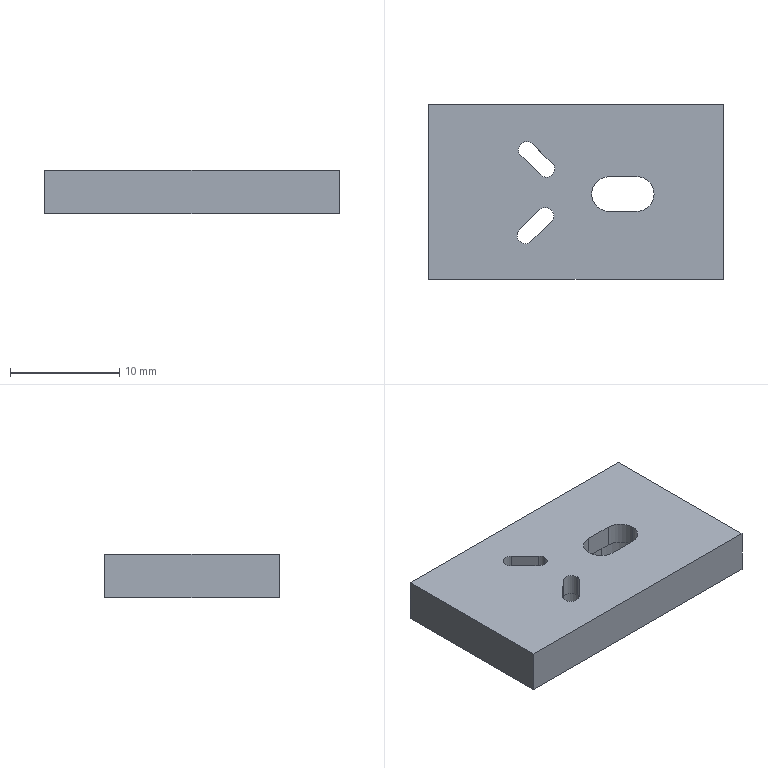Part | SolidWorks | features Cut 2, Extrusion 1, ICE 1 | 1 solid | 39 faces | box 27 x 16 x 4 mm | volume 1564 mm3 | plane 21 | cylinder 18 | commonest cylinder face diameters 1.5 x6 2.5 x6 3.18 x3 5 x3
STEP:
#1=CARTESIAN_POINT('',(4.433,-4.071,2.));
#2=VERTEX_POINT('',#1);
#3=CARTESIAN_POINT('',(6.931,-1.571,2.));
#4=VERTEX_POINT('',#3);
#5=CARTESIAN_POINT('',(6.933,-4.071,2.));
#6=DIRECTION('',(0.,0.,-1.));
#7=DIRECTION('',(-1.,0.,0.));
#8=AXIS2_PLACEMENT_3D('',#5,#6,#7);
#9=CIRCLE('',#8,2.5);
#10=EDGE_CURVE('',#2,#4,#9,.T.);
#11=ORIENTED_EDGE('',*,*,#10,.F.);
#12=CARTESIAN_POINT('',(4.433,-4.071,0.));
#13=VERTEX_POINT('',#12);
#14=CARTESIAN_POINT('',(4.433,-4.071,2.));
#15=DIRECTION('',(0.,0.,-1.));
#16=VECTOR('',#15,1000.);
#17=LINE('',#14,#16);
#18=EDGE_CURVE('',#2,#13,#17,.T.);
#19=ORIENTED_EDGE('',*,*,#18,.T.);
#20=CARTESIAN_POINT('',(6.931,-1.571,0.));
#21=VERTEX_POINT('',#20);
#22=CARTESIAN_POINT('',(6.933,-4.071,0.));
#23=DIRECTION('',(0.,0.,-1.));
#24=DIRECTION('',(-1.,0.,0.));
#25=AXIS2_PLACEMENT_3D('',#22,#23,#24);
#26=CIRCLE('',#25,2.5);
#27=EDGE_CURVE('',#13,#21,#26,.T.);
#28=ORIENTED_EDGE('',*,*,#27,.T.);
#29=CARTESIAN_POINT('',(6.931,-1.571,2.));
#30=DIRECTION('',(0.,0.,-1.));
#31=VECTOR('',#30,1000.);
#32=LINE('',#29,#31);
#33=EDGE_CURVE('',#4,#21,#32,.T.);
#34=ORIENTED_EDGE('',*,*,#33,.F.);
#35=EDGE_LOOP('',(#11,#19,#28,#34));
#36=FACE_OUTER_BOUND('',#35,.T.);
#37=CARTESIAN_POINT('',(6.933,-4.071,2.));
#38=DIRECTION('',(0.,0.,-1.));
#39=DIRECTION('',(-1.,0.,0.));
#40=AXIS2_PLACEMENT_3D('',#37,#38,#39);
#41=CYLINDRICAL_SURFACE('',#40,2.5);
#42=ADVANCED_FACE('',(#36),#41,.F.);
#43=CARTESIAN_POINT('',(-2.005,-7.872,2.));
#44=VERTEX_POINT('',#43);
#45=CARTESIAN_POINT('',(-1.624,-6.973,2.));
#46=VERTEX_POINT('',#45);
#47=CARTESIAN_POINT('',(-0.7552,-7.872,2.));
#48=DIRECTION('',(0.,0.,-1.));
#49=DIRECTION('',(-1.,0.,0.));
#50=AXIS2_PLACEMENT_3D('',#47,#48,#49);
#51=CIRCLE('',#50,1.25);
#52=EDGE_CURVE('',#44,#46,#51,.T.);
#53=ORIENTED_EDGE('',*,*,#52,.F.);
#54=CARTESIAN_POINT('',(-2.005,-7.872,0.));
#55=VERTEX_POINT('',#54);
#56=CARTESIAN_POINT('',(-2.005,-7.872,2.));
#57=DIRECTION('',(0.,0.,-1.));
#58=VECTOR('',#57,1000.);
#59=LINE('',#56,#58);
#60=EDGE_CURVE('',#44,#55,#59,.T.);
#61=ORIENTED_EDGE('',*,*,#60,.T.);
#62=CARTESIAN_POINT('',(-1.624,-6.973,0.));
#63=VERTEX_POINT('',#62);
#64=CARTESIAN_POINT('',(-0.7552,-7.872,0.));
#65=DIRECTION('',(0.,0.,-1.));
#66=DIRECTION('',(-1.,0.,0.));
#67=AXIS2_PLACEMENT_3D('',#64,#65,#66);
#68=CIRCLE('',#67,1.25);
#69=EDGE_CURVE('',#55,#63,#68,.T.);
#70=ORIENTED_EDGE('',*,*,#69,.T.);
#71=CARTESIAN_POINT('',(-1.624,-6.973,2.));
#72=DIRECTION('',(0.,0.,-1.));
#73=VECTOR('',#72,1000.);
#74=LINE('',#71,#73);
#75=EDGE_CURVE('',#46,#63,#74,.T.);
#76=ORIENTED_EDGE('',*,*,#75,.F.);
#77=EDGE_LOOP('',(#53,#61,#70,#76));
#78=FACE_OUTER_BOUND('',#77,.T.);
#79=CARTESIAN_POINT('',(-0.7552,-7.872,2.));
#80=DIRECTION('',(0.,0.,-1.));
#81=DIRECTION('',(-1.,0.,0.));
#82=AXIS2_PLACEMENT_3D('',#79,#80,#81);
#83=CYLINDRICAL_SURFACE('',#82,1.25);
#84=ADVANCED_FACE('',(#78),#83,.F.);
#85=CARTESIAN_POINT('',(-1.875,-0.01768,2.));
#86=VERTEX_POINT('',#85);
#87=CARTESIAN_POINT('',(0.2441,0.881,2.));
#88=VERTEX_POINT('',#87);
#89=CARTESIAN_POINT('',(-0.6247,-0.01768,2.));
#90=DIRECTION('',(0.,0.,-1.));
#91=DIRECTION('',(-1.,0.,0.));
#92=AXIS2_PLACEMENT_3D('',#89,#90,#91);
#93=CIRCLE('',#92,1.25);
#94=EDGE_CURVE('',#86,#88,#93,.T.);
#95=ORIENTED_EDGE('',*,*,#94,.F.);
#96=CARTESIAN_POINT('',(-1.875,-0.01768,0.));
#97=VERTEX_POINT('',#96);
#98=CARTESIAN_POINT('',(-1.875,-0.01768,2.));
#99=DIRECTION('',(0.,0.,-1.));
#100=VECTOR('',#99,1000.);
#101=LINE('',#98,#100);
#102=EDGE_CURVE('',#86,#97,#101,.T.);
#103=ORIENTED_EDGE('',*,*,#102,.T.);
#104=CARTESIAN_POINT('',(0.2441,0.881,0.));
#105=VERTEX_POINT('',#104);
#106=CARTESIAN_POINT('',(-0.6247,-0.01768,0.));
#107=DIRECTION('',(0.,0.,-1.));
#108=DIRECTION('',(-1.,0.,0.));
#109=AXIS2_PLACEMENT_3D('',#106,#107,#108);
#110=CIRCLE('',#109,1.25);
#111=EDGE_CURVE('',#97,#105,#110,.T.);
#112=ORIENTED_EDGE('',*,*,#111,.T.);
#113=CARTESIAN_POINT('',(0.2441,0.881,2.));
#114=DIRECTION('',(0.,0.,-1.));
#115=VECTOR('',#114,1000.);
#116=LINE('',#113,#115);
#117=EDGE_CURVE('',#88,#105,#116,.T.);
#118=ORIENTED_EDGE('',*,*,#117,.F.);
#119=EDGE_LOOP('',(#95,#103,#112,#118));
#120=FACE_OUTER_BOUND('',#119,.T.);
#121=CARTESIAN_POINT('',(-0.6247,-0.01768,2.));
#122=DIRECTION('',(0.,0.,-1.));
#123=DIRECTION('',(-1.,0.,0.));
#124=AXIS2_PLACEMENT_3D('',#121,#122,#123);
#125=CYLINDRICAL_SURFACE('',#124,1.25);
#126=ADVANCED_FACE('',(#120),#125,.F.);
#127=CARTESIAN_POINT('',(11.055,-4.07,2.));
#128=VERTEX_POINT('',#127);
#129=CARTESIAN_POINT('',(9.464,-2.48,2.));
#130=VERTEX_POINT('',#129);
#131=CARTESIAN_POINT('',(9.465,-4.07,2.));
#132=DIRECTION('',(0.,0.,1.));
#133=DIRECTION('',(-1.,0.,0.));
#134=AXIS2_PLACEMENT_3D('',#131,#132,#133);
#135=CIRCLE('',#134,1.59);
#136=EDGE_CURVE('',#128,#130,#135,.T.);
#137=ORIENTED_EDGE('',*,*,#136,.F.);
#138=CARTESIAN_POINT('',(11.055,-4.07,4.));
#139=VERTEX_POINT('',#138);
#140=CARTESIAN_POINT('',(11.055,-4.07,-4.497));
#141=DIRECTION('',(0.,0.,1.));
#142=VECTOR('',#141,1000.);
#143=LINE('',#140,#142);
#144=EDGE_CURVE('',#128,#139,#143,.T.);
#145=ORIENTED_EDGE('',*,*,#144,.T.);
#146=CARTESIAN_POINT('',(9.464,-2.48,4.));
#147=VERTEX_POINT('',#146);
#148=CARTESIAN_POINT('',(9.465,-4.07,4.));
#149=DIRECTION('',(0.,0.,1.));
#150=DIRECTION('',(1.,0.,0.));
#151=AXIS2_PLACEMENT_3D('',#148,#149,#150);
#152=CIRCLE('',#151,1.59);
#153=EDGE_CURVE('',#139,#147,#152,.T.);
#154=ORIENTED_EDGE('',*,*,#153,.T.);
#155=CARTESIAN_POINT('',(9.464,-2.48,-5.208));
#156=DIRECTION('',(0.,0.,1.));
#157=VECTOR('',#156,1000.);
#158=LINE('',#155,#157);
#159=EDGE_CURVE('',#130,#147,#158,.T.);
#160=ORIENTED_EDGE('',*,*,#159,.F.);
#161=EDGE_LOOP('',(#137,#145,#154,#160));
#162=FACE_OUTER_BOUND('',#161,.T.);
#163=CARTESIAN_POINT('',(9.465,-4.07,-4.497));
#164=DIRECTION('',(0.,0.,1.));
#165=DIRECTION('',(1.,0.,0.));
#166=AXIS2_PLACEMENT_3D('',#163,#164,#165);
#167=CYLINDRICAL_SURFACE('',#166,1.59);
#168=ADVANCED_FACE('',(#162),#167,.F.);
#169=CARTESIAN_POINT('',(1.95,-1.782,2.));
#170=VERTEX_POINT('',#169);
#171=CARTESIAN_POINT('',(1.721,-1.242,2.));
#172=VERTEX_POINT('',#171);
#173=CARTESIAN_POINT('',(1.2,-1.782,2.));
#174=DIRECTION('',(0.,0.,1.));
#175=DIRECTION('',(-1.,0.,0.));
#176=AXIS2_PLACEMENT_3D('',#173,#174,#175);
#177=CIRCLE('',#176,0.75);
#178=EDGE_CURVE('',#170,#172,#177,.T.);
#179=ORIENTED_EDGE('',*,*,#178,.F.);
#180=CARTESIAN_POINT('',(1.95,-1.782,4.));
#181=VERTEX_POINT('',#180);
#182=CARTESIAN_POINT('',(1.95,-1.782,-4.497));
#183=DIRECTION('',(0.,0.,1.));
#184=VECTOR('',#183,1000.);
#185=LINE('',#182,#184);
#186=EDGE_CURVE('',#170,#181,#185,.T.);
#187=ORIENTED_EDGE('',*,*,#186,.T.);
#188=CARTESIAN_POINT('',(1.721,-1.242,4.));
#189=VERTEX_POINT('',#188);
#190=CARTESIAN_POINT('',(1.2,-1.782,4.));
#191=DIRECTION('',(0.,0.,1.));
#192=DIRECTION('',(1.,0.,0.));
#193=AXIS2_PLACEMENT_3D('',#190,#191,#192);
#194=CIRCLE('',#193,0.75);
#195=EDGE_CURVE('',#181,#189,#194,.T.);
#196=ORIENTED_EDGE('',*,*,#195,.T.);
#197=CARTESIAN_POINT('',(1.721,-1.242,-5.208));
#198=DIRECTION('',(0.,0.,1.));
#199=VECTOR('',#198,1000.);
#200=LINE('',#197,#199);
#201=EDGE_CURVE('',#172,#189,#200,.T.);
#202=ORIENTED_EDGE('',*,*,#201,.F.);
#203=EDGE_LOOP('',(#179,#187,#196,#202));
#204=FACE_OUTER_BOUND('',#203,.T.);
#205=CARTESIAN_POINT('',(1.2,-1.782,-4.497));
#206=DIRECTION('',(0.,0.,1.));
#207=DIRECTION('',(1.,0.,0.));
#208=AXIS2_PLACEMENT_3D('',#205,#206,#207);
#209=CYLINDRICAL_SURFACE('',#208,0.75);
#210=ADVANCED_FACE('',(#204),#209,.F.);
#211=CARTESIAN_POINT('',(1.873,-6.057,2.));
#212=VERTEX_POINT('',#211);
#213=CARTESIAN_POINT('',(0.6012,-5.518,2.));
#214=VERTEX_POINT('',#213);
#215=CARTESIAN_POINT('',(1.123,-6.057,2.));
#216=DIRECTION('',(0.,0.,1.));
#217=DIRECTION('',(-1.,0.,0.));
#218=AXIS2_PLACEMENT_3D('',#215,#216,#217);
#219=CIRCLE('',#218,0.75);
#220=EDGE_CURVE('',#212,#214,#219,.T.);
#221=ORIENTED_EDGE('',*,*,#220,.F.);
#222=CARTESIAN_POINT('',(1.873,-6.057,4.));
#223=VERTEX_POINT('',#222);
#224=CARTESIAN_POINT('',(1.873,-6.057,-4.497));
#225=DIRECTION('',(0.,0.,1.));
#226=VECTOR('',#225,1000.);
#227=LINE('',#224,#226);
#228=EDGE_CURVE('',#212,#223,#227,.T.);
#229=ORIENTED_EDGE('',*,*,#228,.T.);
#230=CARTESIAN_POINT('',(0.6012,-5.518,4.));
#231=VERTEX_POINT('',#230);
#232=CARTESIAN_POINT('',(1.123,-6.057,4.));
#233=DIRECTION('',(0.,0.,1.));
#234=DIRECTION('',(1.,0.,0.));
#235=AXIS2_PLACEMENT_3D('',#232,#233,#234);
#236=CIRCLE('',#235,0.75);
#237=EDGE_CURVE('',#223,#231,#236,.T.);
#238=ORIENTED_EDGE('',*,*,#237,.T.);
#239=CARTESIAN_POINT('',(0.6012,-5.518,-5.208));
#240=DIRECTION('',(0.,0.,1.));
#241=VECTOR('',#240,1000.);
#242=LINE('',#239,#241);
#243=EDGE_CURVE('',#214,#231,#242,.T.);
#244=ORIENTED_EDGE('',*,*,#243,.F.);
#245=EDGE_LOOP('',(#221,#229,#238,#244));
#246=FACE_OUTER_BOUND('',#245,.T.);
#247=CARTESIAN_POINT('',(1.123,-6.057,-4.497));
#248=DIRECTION('',(0.,0.,1.));
#249=DIRECTION('',(1.,0.,0.));
#250=AXIS2_PLACEMENT_3D('',#247,#248,#249);
#251=CYLINDRICAL_SURFACE('',#250,0.75);
#252=ADVANCED_FACE('',(#246),#251,.F.);
#253=ORIENTED_EDGE('',*,*,#228,.F.);
#254=CARTESIAN_POINT('',(1.644,-6.596,2.));
#255=VERTEX_POINT('',#254);
#256=CARTESIAN_POINT('',(1.123,-6.057,2.));
#257=DIRECTION('',(0.,0.,1.));
#258=DIRECTION('',(-1.,0.,0.));
#259=AXIS2_PLACEMENT_3D('',#256,#257,#258);
#260=CIRCLE('',#259,0.75);
#261=EDGE_CURVE('',#255,#212,#260,.T.);
#262=ORIENTED_EDGE('',*,*,#261,.F.);
#263=CARTESIAN_POINT('',(1.644,-6.596,4.));
#264=VERTEX_POINT('',#263);
#265=CARTESIAN_POINT('',(1.644,-6.596,-5.208));
#266=DIRECTION('',(0.,0.,1.));
#267=VECTOR('',#266,1000.);
#268=LINE('',#265,#267);
#269=EDGE_CURVE('',#255,#264,#268,.T.);
#270=ORIENTED_EDGE('',*,*,#269,.T.);
#271=CARTESIAN_POINT('',(1.123,-6.057,4.));
#272=DIRECTION('',(0.,0.,1.));
#273=DIRECTION('',(1.,0.,0.));
#274=AXIS2_PLACEMENT_3D('',#271,#272,#273);
#275=CIRCLE('',#274,0.75);
#276=EDGE_CURVE('',#264,#223,#275,.T.);
#277=ORIENTED_EDGE('',*,*,#276,.T.);
#278=EDGE_LOOP('',(#253,#262,#270,#277));
#279=FACE_OUTER_BOUND('',#278,.T.);
#280=CARTESIAN_POINT('',(1.123,-6.057,-4.497));
#281=DIRECTION('',(0.,0.,1.));
#282=DIRECTION('',(1.,0.,0.));
#283=AXIS2_PLACEMENT_3D('',#280,#281,#282);
#284=CYLINDRICAL_SURFACE('',#283,0.75);
#285=ADVANCED_FACE('',(#279),#284,.F.);
#286=ORIENTED_EDGE('',*,*,#186,.F.);
#287=CARTESIAN_POINT('',(0.6786,-2.321,2.));
#288=VERTEX_POINT('',#287);
#289=CARTESIAN_POINT('',(1.2,-1.782,2.));
#290=DIRECTION('',(0.,0.,1.));
#291=DIRECTION('',(-1.,0.,0.));
#292=AXIS2_PLACEMENT_3D('',#289,#290,#291);
#293=CIRCLE('',#292,0.75);
#294=EDGE_CURVE('',#288,#170,#293,.T.);
#295=ORIENTED_EDGE('',*,*,#294,.F.);
#296=CARTESIAN_POINT('',(0.6786,-2.321,4.));
#297=VERTEX_POINT('',#296);
#298=CARTESIAN_POINT('',(0.6786,-2.321,-5.208));
#299=DIRECTION('',(0.,0.,1.));
#300=VECTOR('',#299,1000.);
#301=LINE('',#298,#300);
#302=EDGE_CURVE('',#288,#297,#301,.T.);
#303=ORIENTED_EDGE('',*,*,#302,.T.);
#304=CARTESIAN_POINT('',(1.2,-1.782,4.));
#305=DIRECTION('',(0.,0.,1.));
#306=DIRECTION('',(1.,0.,0.));
#307=AXIS2_PLACEMENT_3D('',#304,#305,#306);
#308=CIRCLE('',#307,0.75);
#309=EDGE_CURVE('',#297,#181,#308,.T.);
#310=ORIENTED_EDGE('',*,*,#309,.T.);
#311=EDGE_LOOP('',(#286,#295,#303,#310));
#312=FACE_OUTER_BOUND('',#311,.T.);
#313=CARTESIAN_POINT('',(1.2,-1.782,-4.497));
#314=DIRECTION('',(0.,0.,1.));
#315=DIRECTION('',(1.,0.,0.));
#316=AXIS2_PLACEMENT_3D('',#313,#314,#315);
#317=CYLINDRICAL_SURFACE('',#316,0.75);
#318=ADVANCED_FACE('',(#312),#317,.F.);
#319=ORIENTED_EDGE('',*,*,#144,.F.);
#320=CARTESIAN_POINT('',(9.467,-5.66,2.));
#321=VERTEX_POINT('',#320);
#322=CARTESIAN_POINT('',(9.465,-4.07,2.));
#323=DIRECTION('',(0.,0.,1.));
#324=DIRECTION('',(-1.,0.,0.));
#325=AXIS2_PLACEMENT_3D('',#322,#323,#324);
#326=CIRCLE('',#325,1.59);
#327=EDGE_CURVE('',#321,#128,#326,.T.);
#328=ORIENTED_EDGE('',*,*,#327,.F.);
#329=CARTESIAN_POINT('',(9.467,-5.66,4.));
#330=VERTEX_POINT('',#329);
#331=CARTESIAN_POINT('',(9.467,-5.66,-5.208));
#332=DIRECTION('',(0.,0.,1.));
#333=VECTOR('',#332,1000.);
#334=LINE('',#331,#333);
#335=EDGE_CURVE('',#321,#330,#334,.T.);
#336=ORIENTED_EDGE('',*,*,#335,.T.);
#337=CARTESIAN_POINT('',(9.465,-4.07,4.));
#338=DIRECTION('',(0.,0.,1.));
#339=DIRECTION('',(1.,0.,0.));
#340=AXIS2_PLACEMENT_3D('',#337,#338,#339);
#341=CIRCLE('',#340,1.59);
#342=EDGE_CURVE('',#330,#139,#341,.T.);
#343=ORIENTED_EDGE('',*,*,#342,.T.);
#344=EDGE_LOOP('',(#319,#328,#336,#343));
#345=FACE_OUTER_BOUND('',#344,.T.);
#346=CARTESIAN_POINT('',(9.465,-4.07,-4.497));
#347=DIRECTION('',(0.,0.,1.));
#348=DIRECTION('',(1.,0.,0.));
#349=AXIS2_PLACEMENT_3D('',#346,#347,#348);
#350=CYLINDRICAL_SURFACE('',#349,1.59);
#351=ADVANCED_FACE('',(#345),#350,.F.);
#352=CARTESIAN_POINT('',(6.932,-2.481,2.));
#353=VERTEX_POINT('',#352);
#354=CARTESIAN_POINT('',(6.934,-5.661,2.));
#355=VERTEX_POINT('',#354);
#356=CARTESIAN_POINT('',(6.933,-4.071,2.));
#357=DIRECTION('',(0.,0.,1.));
#358=DIRECTION('',(-1.,0.,0.));
#359=AXIS2_PLACEMENT_3D('',#356,#357,#358);
#360=CIRCLE('',#359,1.59);
#361=EDGE_CURVE('',#353,#355,#360,.T.);
#362=ORIENTED_EDGE('',*,*,#361,.F.);
#363=CARTESIAN_POINT('',(6.932,-2.481,4.));
#364=VERTEX_POINT('',#363);
#365=CARTESIAN_POINT('',(6.932,-2.481,-5.208));
#366=DIRECTION('',(0.,0.,1.));
#367=VECTOR('',#366,1000.);
#368=LINE('',#365,#367);
#369=EDGE_CURVE('',#353,#364,#368,.T.);
#370=ORIENTED_EDGE('',*,*,#369,.T.);
#371=CARTESIAN_POINT('',(6.934,-5.661,4.));
#372=VERTEX_POINT('',#371);
#373=CARTESIAN_POINT('',(6.933,-4.071,4.));
#374=DIRECTION('',(0.,0.,1.));
#375=DIRECTION('',(1.,0.,0.));
#376=AXIS2_PLACEMENT_3D('',#373,#374,#375);
#377=CIRCLE('',#376,1.59);
#378=EDGE_CURVE('',#364,#372,#377,.T.);
#379=ORIENTED_EDGE('',*,*,#378,.T.);
#380=CARTESIAN_POINT('',(6.934,-5.661,-5.208));
#381=DIRECTION('',(0.,0.,1.));
#382=VECTOR('',#381,1000.);
#383=LINE('',#380,#382);
#384=EDGE_CURVE('',#355,#372,#383,.T.);
#385=ORIENTED_EDGE('',*,*,#384,.F.);
#386=EDGE_LOOP('',(#362,#370,#379,#385));
#387=FACE_OUTER_BOUND('',#386,.T.);
#388=CARTESIAN_POINT('',(6.933,-4.071,-5.208));
#389=DIRECTION('',(0.,0.,1.));
#390=DIRECTION('',(1.,0.,0.));
#391=AXIS2_PLACEMENT_3D('',#388,#389,#390);
#392=CYLINDRICAL_SURFACE('',#391,1.59);
#393=ADVANCED_FACE('',(#387),#392,.F.);
#394=CARTESIAN_POINT('',(6.932,-2.481,2.));
#395=DIRECTION('',(-1.,-0.0007677,0.));
#396=VECTOR('',#395,1000.);
#397=LINE('',#394,#396);
#398=EDGE_CURVE('',#130,#353,#397,.T.);
#399=ORIENTED_EDGE('',*,*,#398,.F.);
#400=ORIENTED_EDGE('',*,*,#159,.T.);
#401=CARTESIAN_POINT('',(6.932,-2.481,4.));
#402=DIRECTION('',(-1.,-0.0007677,0.));
#403=VECTOR('',#402,1000.);
#404=LINE('',#401,#403);
#405=EDGE_CURVE('',#147,#364,#404,.T.);
#406=ORIENTED_EDGE('',*,*,#405,.T.);
#407=ORIENTED_EDGE('',*,*,#369,.F.);
#408=EDGE_LOOP('',(#399,#400,#406,#407));
#409=FACE_OUTER_BOUND('',#408,.T.);
#410=CARTESIAN_POINT('',(6.932,-2.481,-5.208));
#411=DIRECTION('',(-0.0007677,1.,0.));
#412=DIRECTION('',(-1.,-0.0007677,0.));
#413=AXIS2_PLACEMENT_3D('',#410,#411,#412);
#414=PLANE('',#413);
#415=ADVANCED_FACE('',(#409),#414,.F.);
#416=CARTESIAN_POINT('',(6.934,-5.661,2.));
#417=DIRECTION('',(1.,0.0007677,0.));
#418=VECTOR('',#417,1000.);
#419=LINE('',#416,#418);
#420=EDGE_CURVE('',#355,#321,#419,.T.);
#421=ORIENTED_EDGE('',*,*,#420,.F.);
#422=ORIENTED_EDGE('',*,*,#384,.T.);
#423=CARTESIAN_POINT('',(6.934,-5.661,4.));
#424=DIRECTION('',(1.,0.0007677,0.));
#425=VECTOR('',#424,1000.);
#426=LINE('',#423,#425);
#427=EDGE_CURVE('',#372,#330,#426,.T.);
#428=ORIENTED_EDGE('',*,*,#427,.T.);
#429=ORIENTED_EDGE('',*,*,#335,.F.);
#430=EDGE_LOOP('',(#421,#422,#428,#429));
#431=FACE_OUTER_BOUND('',#430,.T.);
#432=CARTESIAN_POINT('',(6.934,-5.661,-5.208));
#433=DIRECTION('',(0.0007677,-1.,0.));
#434=DIRECTION('',(1.,0.0007677,0.));
#435=AXIS2_PLACEMENT_3D('',#432,#433,#434);
#436=PLANE('',#435);
#437=ADVANCED_FACE('',(#431),#436,.F.);
#438=CARTESIAN_POINT('',(-0.2339,-8.411,2.));
#439=VERTEX_POINT('',#438);
#440=CARTESIAN_POINT('',(1.644,-6.596,2.));
#441=DIRECTION('',(0.719,0.695,0.));
#442=VECTOR('',#441,1000.);
#443=LINE('',#440,#442);
#444=EDGE_CURVE('',#439,#255,#443,.T.);
#445=ORIENTED_EDGE('',*,*,#444,.F.);
#446=CARTESIAN_POINT('',(-0.2339,-8.411,4.));
#447=VERTEX_POINT('',#446);
#448=CARTESIAN_POINT('',(-0.2339,-8.411,-5.208));
#449=DIRECTION('',(0.,0.,1.));
#450=VECTOR('',#449,1000.);
#451=LINE('',#448,#450);
#452=EDGE_CURVE('',#439,#447,#451,.T.);
#453=ORIENTED_EDGE('',*,*,#452,.T.);
#454=CARTESIAN_POINT('',(1.644,-6.596,4.));
#455=DIRECTION('',(0.719,0.695,0.));
#456=VECTOR('',#455,1000.);
#457=LINE('',#454,#456);
#458=EDGE_CURVE('',#447,#264,#457,.T.);
#459=ORIENTED_EDGE('',*,*,#458,.T.);
#460=ORIENTED_EDGE('',*,*,#269,.F.);
#461=EDGE_LOOP('',(#445,#453,#459,#460));
#462=FACE_OUTER_BOUND('',#461,.T.);
#463=CARTESIAN_POINT('',(1.644,-6.596,-5.208));
#464=DIRECTION('',(0.695,-0.719,0.));
#465=DIRECTION('',(0.719,0.695,0.));
#466=AXIS2_PLACEMENT_3D('',#463,#464,#465);
#467=PLANE('',#466);
#468=ADVANCED_FACE('',(#462),#467,.F.);
#469=CARTESIAN_POINT('',(-1.276,-7.333,2.));
#470=VERTEX_POINT('',#469);
#471=CARTESIAN_POINT('',(-0.7552,-7.872,2.));
#472=DIRECTION('',(0.,0.,1.));
#473=DIRECTION('',(-1.,0.,0.));
#474=AXIS2_PLACEMENT_3D('',#471,#472,#473);
#475=CIRCLE('',#474,0.75);
#476=EDGE_CURVE('',#470,#439,#475,.T.);
#477=ORIENTED_EDGE('',*,*,#476,.F.);
#478=CARTESIAN_POINT('',(-1.276,-7.333,4.));
#479=VERTEX_POINT('',#478);
#480=CARTESIAN_POINT('',(-1.276,-7.333,-5.208));
#481=DIRECTION('',(0.,0.,1.));
#482=VECTOR('',#481,1000.);
#483=LINE('',#480,#482);
#484=EDGE_CURVE('',#470,#479,#483,.T.);
#485=ORIENTED_EDGE('',*,*,#484,.T.);
#486=CARTESIAN_POINT('',(-0.7552,-7.872,4.));
#487=DIRECTION('',(0.,0.,1.));
#488=DIRECTION('',(1.,0.,0.));
#489=AXIS2_PLACEMENT_3D('',#486,#487,#488);
#490=CIRCLE('',#489,0.75);
#491=EDGE_CURVE('',#479,#447,#490,.T.);
#492=ORIENTED_EDGE('',*,*,#491,.T.);
#493=ORIENTED_EDGE('',*,*,#452,.F.);
#494=EDGE_LOOP('',(#477,#485,#492,#493));
#495=FACE_OUTER_BOUND('',#494,.T.);
#496=CARTESIAN_POINT('',(-0.7552,-7.872,-5.208));
#497=DIRECTION('',(0.,0.,1.));
#498=DIRECTION('',(1.,0.,0.));
#499=AXIS2_PLACEMENT_3D('',#496,#497,#498);
#500=CYLINDRICAL_SURFACE('',#499,0.75);
#501=ADVANCED_FACE('',(#495),#500,.F.);
#502=CARTESIAN_POINT('',(-1.276,-7.333,2.));
#503=DIRECTION('',(-0.719,-0.695,0.));
#504=VECTOR('',#503,1000.);
#505=LINE('',#502,#504);
#506=EDGE_CURVE('',#214,#470,#505,.T.);
#507=ORIENTED_EDGE('',*,*,#506,.F.);
#508=ORIENTED_EDGE('',*,*,#243,.T.);
#509=CARTESIAN_POINT('',(-1.276,-7.333,4.));
#510=DIRECTION('',(-0.719,-0.695,0.));
#511=VECTOR('',#510,1000.);
#512=LINE('',#509,#511);
#513=EDGE_CURVE('',#231,#479,#512,.T.);
#514=ORIENTED_EDGE('',*,*,#513,.T.);
#515=ORIENTED_EDGE('',*,*,#484,.F.);
#516=EDGE_LOOP('',(#507,#508,#514,#515));
#517=FACE_OUTER_BOUND('',#516,.T.);
#518=CARTESIAN_POINT('',(-1.276,-7.333,-5.208));
#519=DIRECTION('',(-0.695,0.719,0.));
#520=DIRECTION('',(-0.719,-0.695,0.));
#521=AXIS2_PLACEMENT_3D('',#518,#519,#520);
#522=PLANE('',#521);
#523=ADVANCED_FACE('',(#517),#522,.F.);
#524=CARTESIAN_POINT('',(-0.1034,0.5215,2.));
#525=VERTEX_POINT('',#524);
#526=CARTESIAN_POINT('',(-1.146,-0.5569,2.));
#527=VERTEX_POINT('',#526);
#528=CARTESIAN_POINT('',(-0.6247,-0.01768,2.));
#529=DIRECTION('',(0.,0.,1.));
#530=DIRECTION('',(-1.,0.,0.));
#531=AXIS2_PLACEMENT_3D('',#528,#529,#530);
#532=CIRCLE('',#531,0.75);
#533=EDGE_CURVE('',#525,#527,#532,.T.);
#534=ORIENTED_EDGE('',*,*,#533,.F.);
#535=CARTESIAN_POINT('',(-0.1034,0.5215,4.));
#536=VERTEX_POINT('',#535);
#537=CARTESIAN_POINT('',(-0.1034,0.5215,-5.208));
#538=DIRECTION('',(0.,0.,1.));
#539=VECTOR('',#538,1000.);
#540=LINE('',#537,#539);
#541=EDGE_CURVE('',#525,#536,#540,.T.);
#542=ORIENTED_EDGE('',*,*,#541,.T.);
#543=CARTESIAN_POINT('',(-1.146,-0.5569,4.));
#544=VERTEX_POINT('',#543);
#545=CARTESIAN_POINT('',(-0.6247,-0.01768,4.));
#546=DIRECTION('',(0.,0.,1.));
#547=DIRECTION('',(1.,0.,0.));
#548=AXIS2_PLACEMENT_3D('',#545,#546,#547);
#549=CIRCLE('',#548,0.75);
#550=EDGE_CURVE('',#536,#544,#549,.T.);
#551=ORIENTED_EDGE('',*,*,#550,.T.);
#552=CARTESIAN_POINT('',(-1.146,-0.5569,-5.208));
#553=DIRECTION('',(0.,0.,1.));
#554=VECTOR('',#553,1000.);
#555=LINE('',#552,#554);
#556=EDGE_CURVE('',#527,#544,#555,.T.);
#557=ORIENTED_EDGE('',*,*,#556,.F.);
#558=EDGE_LOOP('',(#534,#542,#551,#557));
#559=FACE_OUTER_BOUND('',#558,.T.);
#560=CARTESIAN_POINT('',(-0.6247,-0.01768,-5.208));
#561=DIRECTION('',(0.,0.,1.));
#562=DIRECTION('',(1.,0.,0.));
#563=AXIS2_PLACEMENT_3D('',#560,#561,#562);
#564=CYLINDRICAL_SURFACE('',#563,0.75);
#565=ADVANCED_FACE('',(#559),#564,.F.);
#566=CARTESIAN_POINT('',(1.721,-1.242,2.));
#567=DIRECTION('',(-0.719,0.695,0.));
#568=VECTOR('',#567,1000.);
#569=LINE('',#566,#568);
#570=EDGE_CURVE('',#172,#525,#569,.T.);
#571=ORIENTED_EDGE('',*,*,#570,.F.);
#572=ORIENTED_EDGE('',*,*,#201,.T.);
#573=CARTESIAN_POINT('',(1.721,-1.242,4.));
#574=DIRECTION('',(-0.719,0.695,0.));
#575=VECTOR('',#574,1000.);
#576=LINE('',#573,#575);
#577=EDGE_CURVE('',#189,#536,#576,.T.);
#578=ORIENTED_EDGE('',*,*,#577,.T.);
#579=ORIENTED_EDGE('',*,*,#541,.F.);
#580=EDGE_LOOP('',(#571,#572,#578,#579));
#581=FACE_OUTER_BOUND('',#580,.T.);
#582=CARTESIAN_POINT('',(1.721,-1.242,-5.208));
#583=DIRECTION('',(0.695,0.719,0.));
#584=DIRECTION('',(-0.719,0.695,0.));
#585=AXIS2_PLACEMENT_3D('',#582,#583,#584);
#586=PLANE('',#585);
#587=ADVANCED_FACE('',(#581),#586,.F.);
#588=CARTESIAN_POINT('',(-1.146,-0.5569,2.));
#589=DIRECTION('',(0.719,-0.695,0.));
#590=VECTOR('',#589,1000.);
#591=LINE('',#588,#590);
#592=EDGE_CURVE('',#527,#288,#591,.T.);
#593=ORIENTED_EDGE('',*,*,#592,.F.);
#594=ORIENTED_EDGE('',*,*,#556,.T.);
#595=CARTESIAN_POINT('',(-1.146,-0.5569,4.));
#596=DIRECTION('',(0.719,-0.695,0.));
#597=VECTOR('',#596,1000.);
#598=LINE('',#595,#597);
#599=EDGE_CURVE('',#544,#297,#598,.T.);
#600=ORIENTED_EDGE('',*,*,#599,.T.);
#601=ORIENTED_EDGE('',*,*,#302,.F.);
#602=EDGE_LOOP('',(#593,#594,#600,#601));
#603=FACE_OUTER_BOUND('',#602,.T.);
#604=CARTESIAN_POINT('',(-1.146,-0.5569,-5.208));
#605=DIRECTION('',(-0.695,-0.719,0.));
#606=DIRECTION('',(0.719,-0.695,0.));
#607=AXIS2_PLACEMENT_3D('',#604,#605,#606);
#608=PLANE('',#607);
#609=ADVANCED_FACE('',(#603),#608,.F.);
#610=CARTESIAN_POINT('',(-9.601,4.118,0.));
#611=VERTEX_POINT('',#610);
#612=CARTESIAN_POINT('',(-9.601,-11.882,0.));
#613=VERTEX_POINT('',#612);
#614=CARTESIAN_POINT('',(-9.601,4.118,0.));
#615=DIRECTION('',(0.,-1.,0.));
#616=VECTOR('',#615,1000.);
#617=LINE('',#614,#616);
#618=EDGE_CURVE('',#611,#613,#617,.T.);
#619=ORIENTED_EDGE('',*,*,#618,.T.);
#620=CARTESIAN_POINT('',(-9.601,-11.882,4.));
#621=VERTEX_POINT('',#620);
#622=CARTESIAN_POINT('',(-9.601,-11.882,4.));
#623=DIRECTION('',(0.,0.,-1.));
#624=VECTOR('',#623,1000.);
#625=LINE('',#622,#624);
#626=EDGE_CURVE('',#621,#613,#625,.T.);
#627=ORIENTED_EDGE('',*,*,#626,.F.);
#628=CARTESIAN_POINT('',(-9.601,4.118,4.));
#629=VERTEX_POINT('',#628);
#630=CARTESIAN_POINT('',(-9.601,4.118,4.));
#631=DIRECTION('',(0.,-1.,0.));
#632=VECTOR('',#631,1000.);
#633=LINE('',#630,#632);
#634=EDGE_CURVE('',#629,#621,#633,.T.);
#635=ORIENTED_EDGE('',*,*,#634,.F.);
#636=CARTESIAN_POINT('',(-9.601,4.118,4.));
#637=DIRECTION('',(0.,0.,-1.));
#638=VECTOR('',#637,1000.);
#639=LINE('',#636,#638);
#640=EDGE_CURVE('',#629,#611,#639,.T.);
#641=ORIENTED_EDGE('',*,*,#640,.T.);
#642=EDGE_LOOP('',(#619,#627,#635,#641));
#643=FACE_OUTER_BOUND('',#642,.T.);
#644=CARTESIAN_POINT('',(-9.601,4.118,4.));
#645=DIRECTION('',(1.,0.,0.));
#646=DIRECTION('',(0.,1.,0.));
#647=AXIS2_PLACEMENT_3D('',#644,#645,#646);
#648=PLANE('',#647);
#649=ADVANCED_FACE('',(#643),#648,.F.);
#650=CARTESIAN_POINT('',(17.399,-11.882,0.));
#651=VERTEX_POINT('',#650);
#652=CARTESIAN_POINT('',(-9.601,-11.882,0.));
#653=DIRECTION('',(1.,0.,0.));
#654=VECTOR('',#653,1000.);
#655=LINE('',#652,#654);
#656=EDGE_CURVE('',#613,#651,#655,.T.);
#657=ORIENTED_EDGE('',*,*,#656,.T.);
#658=CARTESIAN_POINT('',(17.399,-11.882,4.));
#659=VERTEX_POINT('',#658);
#660=CARTESIAN_POINT('',(17.399,-11.882,4.));
#661=DIRECTION('',(0.,0.,-1.));
#662=VECTOR('',#661,1000.);
#663=LINE('',#660,#662);
#664=EDGE_CURVE('',#659,#651,#663,.T.);
#665=ORIENTED_EDGE('',*,*,#664,.F.);
#666=CARTESIAN_POINT('',(-9.601,-11.882,4.));
#667=DIRECTION('',(1.,0.,0.));
#668=VECTOR('',#667,1000.);
#669=LINE('',#666,#668);
#670=EDGE_CURVE('',#621,#659,#669,.T.);
#671=ORIENTED_EDGE('',*,*,#670,.F.);
#672=ORIENTED_EDGE('',*,*,#626,.T.);
#673=EDGE_LOOP('',(#657,#665,#671,#672));
#674=FACE_OUTER_BOUND('',#673,.T.);
#675=CARTESIAN_POINT('',(-9.601,-11.882,4.));
#676=DIRECTION('',(0.,1.,0.));
#677=DIRECTION('',(0.,0.,1.));
#678=AXIS2_PLACEMENT_3D('',#675,#676,#677);
#679=PLANE('',#678);
#680=ADVANCED_FACE('',(#674),#679,.F.);
#681=CARTESIAN_POINT('',(17.399,4.118,0.));
#682=VERTEX_POINT('',#681);
#683=CARTESIAN_POINT('',(17.399,4.118,0.));
#684=DIRECTION('',(0.,1.,0.));
#685=VECTOR('',#684,1000.);
#686=LINE('',#683,#685);
#687=EDGE_CURVE('',#651,#682,#686,.T.);
#688=ORIENTED_EDGE('',*,*,#687,.T.);
#689=CARTESIAN_POINT('',(17.399,4.118,4.));
#690=VERTEX_POINT('',#689);
#691=CARTESIAN_POINT('',(17.399,4.118,4.));
#692=DIRECTION('',(0.,0.,-1.));
#693=VECTOR('',#692,1000.);
#694=LINE('',#691,#693);
#695=EDGE_CURVE('',#690,#682,#694,.T.);
#696=ORIENTED_EDGE('',*,*,#695,.F.);
#697=CARTESIAN_POINT('',(17.399,4.118,4.));
#698=DIRECTION('',(0.,1.,0.));
#699=VECTOR('',#698,1000.);
#700=LINE('',#697,#699);
#701=EDGE_CURVE('',#659,#690,#700,.T.);
#702=ORIENTED_EDGE('',*,*,#701,.F.);
#703=ORIENTED_EDGE('',*,*,#664,.T.);
#704=EDGE_LOOP('',(#688,#696,#702,#703));
#705=FACE_OUTER_BOUND('',#704,.T.);
#706=CARTESIAN_POINT('',(17.399,4.118,4.));
#707=DIRECTION('',(-1.,0.,0.));
#708=DIRECTION('',(0.,-1.,0.));
#709=AXIS2_PLACEMENT_3D('',#706,#707,#708);
#710=PLANE('',#709);
#711=ADVANCED_FACE('',(#705),#710,.F.);
#712=CARTESIAN_POINT('',(-9.601,4.118,0.));
#713=DIRECTION('',(-1.,0.,0.));
#714=VECTOR('',#713,1000.);
#715=LINE('',#712,#714);
#716=EDGE_CURVE('',#682,#611,#715,.T.);
#717=ORIENTED_EDGE('',*,*,#716,.T.);
#718=ORIENTED_EDGE('',*,*,#640,.F.);
#719=CARTESIAN_POINT('',(-9.601,4.118,4.));
#720=DIRECTION('',(-1.,0.,0.));
#721=VECTOR('',#720,1000.);
#722=LINE('',#719,#721);
#723=EDGE_CURVE('',#690,#629,#722,.T.);
#724=ORIENTED_EDGE('',*,*,#723,.F.);
#725=ORIENTED_EDGE('',*,*,#695,.T.);
#726=EDGE_LOOP('',(#717,#718,#724,#725));
#727=FACE_OUTER_BOUND('',#726,.T.);
#728=CARTESIAN_POINT('',(-9.601,4.118,4.));
#729=DIRECTION('',(0.,-1.,0.));
#730=DIRECTION('',(0.,0.,-1.));
#731=AXIS2_PLACEMENT_3D('',#728,#729,#730);
#732=PLANE('',#731);
#733=ADVANCED_FACE('',(#727),#732,.F.);
#734=ORIENTED_EDGE('',*,*,#577,.F.);
#735=ORIENTED_EDGE('',*,*,#195,.F.);
#736=ORIENTED_EDGE('',*,*,#309,.F.);
#737=ORIENTED_EDGE('',*,*,#599,.F.);
#738=ORIENTED_EDGE('',*,*,#550,.F.);
#739=EDGE_LOOP('',(#734,#735,#736,#737,#738));
#740=FACE_BOUND('',#739,.T.);
#741=ORIENTED_EDGE('',*,*,#405,.F.);
#742=ORIENTED_EDGE('',*,*,#153,.F.);
#743=ORIENTED_EDGE('',*,*,#342,.F.);
#744=ORIENTED_EDGE('',*,*,#427,.F.);
#745=ORIENTED_EDGE('',*,*,#378,.F.);
#746=EDGE_LOOP('',(#741,#742,#743,#744,#745));
#747=FACE_BOUND('',#746,.T.);
#748=ORIENTED_EDGE('',*,*,#458,.F.);
#749=ORIENTED_EDGE('',*,*,#491,.F.);
#750=ORIENTED_EDGE('',*,*,#513,.F.);
#751=ORIENTED_EDGE('',*,*,#237,.F.);
#752=ORIENTED_EDGE('',*,*,#276,.F.);
#753=EDGE_LOOP('',(#748,#749,#750,#751,#752));
#754=FACE_BOUND('',#753,.T.);
#755=ORIENTED_EDGE('',*,*,#634,.T.);
#756=ORIENTED_EDGE('',*,*,#670,.T.);
#757=ORIENTED_EDGE('',*,*,#701,.T.);
#758=ORIENTED_EDGE('',*,*,#723,.T.);
#759=EDGE_LOOP('',(#755,#756,#757,#758));
#760=FACE_OUTER_BOUND('',#759,.T.);
#761=CARTESIAN_POINT('',(0.,0.,4.));
#762=DIRECTION('',(0.,0.,1.));
#763=DIRECTION('',(1.,0.,0.));
#764=AXIS2_PLACEMENT_3D('',#761,#762,#763);
#765=PLANE('',#764);
#766=ADVANCED_FACE('',(#740,#747,#754,#760),#765,.T.);
#767=CARTESIAN_POINT('',(9.463,-1.57,0.));
#768=VERTEX_POINT('',#767);
#769=CARTESIAN_POINT('',(9.463,-1.57,0.));
#770=DIRECTION('',(1.,0.0007677,0.));
#771=VECTOR('',#770,1000.);
#772=LINE('',#769,#771);
#773=EDGE_CURVE('',#21,#768,#772,.T.);
#774=ORIENTED_EDGE('',*,*,#773,.F.);
#775=ORIENTED_EDGE('',*,*,#27,.F.);
#776=CARTESIAN_POINT('',(6.935,-6.571,0.));
#777=VERTEX_POINT('',#776);
#778=CARTESIAN_POINT('',(6.933,-4.071,0.));
#779=DIRECTION('',(0.,0.,-1.));
#780=DIRECTION('',(-1.,0.,0.));
#781=AXIS2_PLACEMENT_3D('',#778,#779,#780);
#782=CIRCLE('',#781,2.5);
#783=EDGE_CURVE('',#777,#13,#782,.T.);
#784=ORIENTED_EDGE('',*,*,#783,.F.);
#785=CARTESIAN_POINT('',(9.467,-6.57,0.));
#786=VERTEX_POINT('',#785);
#787=CARTESIAN_POINT('',(9.467,-6.57,0.));
#788=DIRECTION('',(-1.,-0.0007677,0.));
#789=VECTOR('',#788,1000.);
#790=LINE('',#787,#789);
#791=EDGE_CURVE('',#786,#777,#790,.T.);
#792=ORIENTED_EDGE('',*,*,#791,.F.);
#793=CARTESIAN_POINT('',(9.465,-4.07,0.));
#794=DIRECTION('',(0.,0.,-1.));
#795=DIRECTION('',(-1.,0.,0.));
#796=AXIS2_PLACEMENT_3D('',#793,#794,#795);
#797=CIRCLE('',#796,2.5);
#798=EDGE_CURVE('',#768,#786,#797,.T.);
#799=ORIENTED_EDGE('',*,*,#798,.F.);
#800=EDGE_LOOP('',(#774,#775,#784,#792,#799));
#801=FACE_BOUND('',#800,.T.);
#802=CARTESIAN_POINT('',(0.2537,-5.158,0.));
#803=VERTEX_POINT('',#802);
#804=CARTESIAN_POINT('',(0.2537,-5.158,0.));
#805=DIRECTION('',(0.719,0.695,0.));
#806=VECTOR('',#805,1000.);
#807=LINE('',#804,#806);
#808=EDGE_CURVE('',#63,#803,#807,.T.);
#809=ORIENTED_EDGE('',*,*,#808,.F.);
#810=ORIENTED_EDGE('',*,*,#69,.F.);
#811=CARTESIAN_POINT('',(0.1136,-8.771,0.));
#812=VERTEX_POINT('',#811);
#813=CARTESIAN_POINT('',(-0.7552,-7.872,0.));
#814=DIRECTION('',(0.,0.,-1.));
#815=DIRECTION('',(-1.,0.,0.));
#816=AXIS2_PLACEMENT_3D('',#813,#814,#815);
#817=CIRCLE('',#816,1.25);
#818=EDGE_CURVE('',#812,#55,#817,.T.);
#819=ORIENTED_EDGE('',*,*,#818,.F.);
#820=CARTESIAN_POINT('',(1.991,-6.955,0.));
#821=VERTEX_POINT('',#820);
#822=CARTESIAN_POINT('',(1.991,-6.955,0.));
#823=DIRECTION('',(-0.719,-0.695,0.));
#824=VECTOR('',#823,1000.);
#825=LINE('',#822,#824);
#826=EDGE_CURVE('',#821,#812,#825,.T.);
#827=ORIENTED_EDGE('',*,*,#826,.F.);
#828=CARTESIAN_POINT('',(1.123,-6.057,0.));
#829=DIRECTION('',(0.,0.,-1.));
#830=DIRECTION('',(-1.,0.,0.));
#831=AXIS2_PLACEMENT_3D('',#828,#829,#830);
#832=CIRCLE('',#831,1.25);
#833=EDGE_CURVE('',#803,#821,#832,.T.);
#834=ORIENTED_EDGE('',*,*,#833,.F.);
#835=EDGE_LOOP('',(#809,#810,#819,#827,#834));
#836=FACE_BOUND('',#835,.T.);
#837=CARTESIAN_POINT('',(2.069,-0.8829,0.));
#838=VERTEX_POINT('',#837);
#839=CARTESIAN_POINT('',(0.2441,0.881,0.));
#840=DIRECTION('',(0.719,-0.695,0.));
#841=VECTOR('',#840,1000.);
#842=LINE('',#839,#841);
#843=EDGE_CURVE('',#105,#838,#842,.T.);
#844=ORIENTED_EDGE('',*,*,#843,.F.);
#845=ORIENTED_EDGE('',*,*,#111,.F.);
#846=CARTESIAN_POINT('',(-1.494,-0.9164,0.));
#847=VERTEX_POINT('',#846);
#848=CARTESIAN_POINT('',(-0.6247,-0.01768,0.));
#849=DIRECTION('',(0.,0.,-1.));
#850=DIRECTION('',(-1.,0.,0.));
#851=AXIS2_PLACEMENT_3D('',#848,#849,#850);
#852=CIRCLE('',#851,1.25);
#853=EDGE_CURVE('',#847,#97,#852,.T.);
#854=ORIENTED_EDGE('',*,*,#853,.F.);
#855=CARTESIAN_POINT('',(0.3311,-2.68,0.));
#856=VERTEX_POINT('',#855);
#857=CARTESIAN_POINT('',(0.3311,-2.68,0.));
#858=DIRECTION('',(-0.719,0.695,0.));
#859=VECTOR('',#858,1000.);
#860=LINE('',#857,#859);
#861=EDGE_CURVE('',#856,#847,#860,.T.);
#862=ORIENTED_EDGE('',*,*,#861,.F.);
#863=CARTESIAN_POINT('',(1.2,-1.782,0.));
#864=DIRECTION('',(0.,0.,-1.));
#865=DIRECTION('',(-1.,0.,0.));
#866=AXIS2_PLACEMENT_3D('',#863,#864,#865);
#867=CIRCLE('',#866,1.25);
#868=EDGE_CURVE('',#838,#856,#867,.T.);
#869=ORIENTED_EDGE('',*,*,#868,.F.);
#870=EDGE_LOOP('',(#844,#845,#854,#862,#869));
#871=FACE_BOUND('',#870,.T.);
#872=ORIENTED_EDGE('',*,*,#618,.F.);
#873=ORIENTED_EDGE('',*,*,#716,.F.);
#874=ORIENTED_EDGE('',*,*,#687,.F.);
#875=ORIENTED_EDGE('',*,*,#656,.F.);
#876=EDGE_LOOP('',(#872,#873,#874,#875));
#877=FACE_OUTER_BOUND('',#876,.T.);
#878=CARTESIAN_POINT('',(0.,0.,0.));
#879=DIRECTION('',(0.,0.,1.));
#880=DIRECTION('',(1.,0.,0.));
#881=AXIS2_PLACEMENT_3D('',#878,#879,#880);
#882=PLANE('',#881);
#883=ADVANCED_FACE('',(#801,#836,#871,#877),#882,.F.);
#884=CARTESIAN_POINT('',(-1.494,-0.9164,2.));
#885=VERTEX_POINT('',#884);
#886=CARTESIAN_POINT('',(-0.6247,-0.01768,2.));
#887=DIRECTION('',(0.,0.,-1.));
#888=DIRECTION('',(-1.,0.,0.));
#889=AXIS2_PLACEMENT_3D('',#886,#887,#888);
#890=CIRCLE('',#889,1.25);
#891=EDGE_CURVE('',#885,#86,#890,.T.);
#892=ORIENTED_EDGE('',*,*,#891,.T.);
#893=ORIENTED_EDGE('',*,*,#94,.T.);
#894=CARTESIAN_POINT('',(2.069,-0.8829,2.));
#895=VERTEX_POINT('',#894);
#896=CARTESIAN_POINT('',(0.2441,0.881,2.));
#897=DIRECTION('',(0.719,-0.695,0.));
#898=VECTOR('',#897,1000.);
#899=LINE('',#896,#898);
#900=EDGE_CURVE('',#88,#895,#899,.T.);
#901=ORIENTED_EDGE('',*,*,#900,.T.);
#902=CARTESIAN_POINT('',(0.3311,-2.68,2.));
#903=VERTEX_POINT('',#902);
#904=CARTESIAN_POINT('',(1.2,-1.782,2.));
#905=DIRECTION('',(0.,0.,-1.));
#906=DIRECTION('',(-1.,0.,0.));
#907=AXIS2_PLACEMENT_3D('',#904,#905,#906);
#908=CIRCLE('',#907,1.25);
#909=EDGE_CURVE('',#895,#903,#908,.T.);
#910=ORIENTED_EDGE('',*,*,#909,.T.);
#911=CARTESIAN_POINT('',(0.3311,-2.68,2.));
#912=DIRECTION('',(-0.719,0.695,0.));
#913=VECTOR('',#912,1000.);
#914=LINE('',#911,#913);
#915=EDGE_CURVE('',#903,#885,#914,.T.);
#916=ORIENTED_EDGE('',*,*,#915,.T.);
#917=EDGE_LOOP('',(#892,#893,#901,#910,#916));
#918=FACE_OUTER_BOUND('',#917,.T.);
#919=ORIENTED_EDGE('',*,*,#570,.T.);
#920=ORIENTED_EDGE('',*,*,#533,.T.);
#921=ORIENTED_EDGE('',*,*,#592,.T.);
#922=ORIENTED_EDGE('',*,*,#294,.T.);
#923=ORIENTED_EDGE('',*,*,#178,.T.);
#924=EDGE_LOOP('',(#919,#920,#921,#922,#923));
#925=FACE_BOUND('',#924,.T.);
#926=CARTESIAN_POINT('',(-0.6247,-0.01768,2.));
#927=DIRECTION('',(0.,0.,-1.));
#928=DIRECTION('',(-1.,0.,0.));
#929=AXIS2_PLACEMENT_3D('',#926,#927,#928);
#930=PLANE('',#929);
#931=ADVANCED_FACE('',(#918,#925),#930,.T.);
#932=ORIENTED_EDGE('',*,*,#102,.F.);
#933=ORIENTED_EDGE('',*,*,#891,.F.);
#934=CARTESIAN_POINT('',(-1.494,-0.9164,2.));
#935=DIRECTION('',(0.,0.,-1.));
#936=VECTOR('',#935,1000.);
#937=LINE('',#934,#936);
#938=EDGE_CURVE('',#885,#847,#937,.T.);
#939=ORIENTED_EDGE('',*,*,#938,.T.);
#940=ORIENTED_EDGE('',*,*,#853,.T.);
#941=EDGE_LOOP('',(#932,#933,#939,#940));
#942=FACE_OUTER_BOUND('',#941,.T.);
#943=CARTESIAN_POINT('',(-0.6247,-0.01768,2.));
#944=DIRECTION('',(0.,0.,-1.));
#945=DIRECTION('',(-1.,0.,0.));
#946=AXIS2_PLACEMENT_3D('',#943,#944,#945);
#947=CYLINDRICAL_SURFACE('',#946,1.25);
#948=ADVANCED_FACE('',(#942),#947,.F.);
#949=ORIENTED_EDGE('',*,*,#861,.T.);
#950=ORIENTED_EDGE('',*,*,#938,.F.);
#951=ORIENTED_EDGE('',*,*,#915,.F.);
#952=CARTESIAN_POINT('',(0.3311,-2.68,2.));
#953=DIRECTION('',(0.,0.,-1.));
#954=VECTOR('',#953,1000.);
#955=LINE('',#952,#954);
#956=EDGE_CURVE('',#903,#856,#955,.T.);
#957=ORIENTED_EDGE('',*,*,#956,.T.);
#958=EDGE_LOOP('',(#949,#950,#951,#957));
#959=FACE_OUTER_BOUND('',#958,.T.);
#960=CARTESIAN_POINT('',(0.3311,-2.68,2.));
#961=DIRECTION('',(-0.695,-0.719,0.));
#962=DIRECTION('',(0.719,-0.695,0.));
#963=AXIS2_PLACEMENT_3D('',#960,#961,#962);
#964=PLANE('',#963);
#965=ADVANCED_FACE('',(#959),#964,.F.);
#966=ORIENTED_EDGE('',*,*,#868,.T.);
#967=ORIENTED_EDGE('',*,*,#956,.F.);
#968=ORIENTED_EDGE('',*,*,#909,.F.);
#969=CARTESIAN_POINT('',(2.069,-0.8829,2.));
#970=DIRECTION('',(0.,0.,-1.));
#971=VECTOR('',#970,1000.);
#972=LINE('',#969,#971);
#973=EDGE_CURVE('',#895,#838,#972,.T.);
#974=ORIENTED_EDGE('',*,*,#973,.T.);
#975=EDGE_LOOP('',(#966,#967,#968,#974));
#976=FACE_OUTER_BOUND('',#975,.T.);
#977=CARTESIAN_POINT('',(1.2,-1.782,2.));
#978=DIRECTION('',(0.,0.,-1.));
#979=DIRECTION('',(-1.,0.,0.));
#980=AXIS2_PLACEMENT_3D('',#977,#978,#979);
#981=CYLINDRICAL_SURFACE('',#980,1.25);
#982=ADVANCED_FACE('',(#976),#981,.F.);
#983=ORIENTED_EDGE('',*,*,#843,.T.);
#984=ORIENTED_EDGE('',*,*,#973,.F.);
#985=ORIENTED_EDGE('',*,*,#900,.F.);
#986=ORIENTED_EDGE('',*,*,#117,.T.);
#987=EDGE_LOOP('',(#983,#984,#985,#986));
#988=FACE_OUTER_BOUND('',#987,.T.);
#989=CARTESIAN_POINT('',(0.2441,0.881,2.));
#990=DIRECTION('',(0.695,0.719,0.));
#991=DIRECTION('',(-0.719,0.695,0.));
#992=AXIS2_PLACEMENT_3D('',#989,#990,#991);
#993=PLANE('',#992);
#994=ADVANCED_FACE('',(#988),#993,.F.);
#995=CARTESIAN_POINT('',(0.1136,-8.771,2.));
#996=VERTEX_POINT('',#995);
#997=CARTESIAN_POINT('',(-0.7552,-7.872,2.));
#998=DIRECTION('',(0.,0.,-1.));
#999=DIRECTION('',(-1.,0.,0.));
#1000=AXIS2_PLACEMENT_3D('',#997,#998,#999);
#1001=CIRCLE('',#1000,1.25);
#1002=EDGE_CURVE('',#996,#44,#1001,.T.);
#1003=ORIENTED_EDGE('',*,*,#1002,.T.);
#1004=ORIENTED_EDGE('',*,*,#52,.T.);
#1005=CARTESIAN_POINT('',(0.2537,-5.158,2.));
#1006=VERTEX_POINT('',#1005);
#1007=CARTESIAN_POINT('',(0.2537,-5.158,2.));
#1008=DIRECTION('',(0.719,0.695,0.));
#1009=VECTOR('',#1008,1000.);
#1010=LINE('',#1007,#1009);
#1011=EDGE_CURVE('',#46,#1006,#1010,.T.);
#1012=ORIENTED_EDGE('',*,*,#1011,.T.);
#1013=CARTESIAN_POINT('',(1.991,-6.955,2.));
#1014=VERTEX_POINT('',#1013);
#1015=CARTESIAN_POINT('',(1.123,-6.057,2.));
#1016=DIRECTION('',(0.,0.,-1.));
#1017=DIRECTION('',(-1.,0.,0.));
#1018=AXIS2_PLACEMENT_3D('',#1015,#1016,#1017);
#1019=CIRCLE('',#1018,1.25);
#1020=EDGE_CURVE('',#1006,#1014,#1019,.T.);
#1021=ORIENTED_EDGE('',*,*,#1020,.T.);
#1022=CARTESIAN_POINT('',(1.991,-6.955,2.));
#1023=DIRECTION('',(-0.719,-0.695,0.));
#1024=VECTOR('',#1023,1000.);
#1025=LINE('',#1022,#1024);
#1026=EDGE_CURVE('',#1014,#996,#1025,.T.);
#1027=ORIENTED_EDGE('',*,*,#1026,.T.);
#1028=EDGE_LOOP('',(#1003,#1004,#1012,#1021,#1027));
#1029=FACE_OUTER_BOUND('',#1028,.T.);
#1030=ORIENTED_EDGE('',*,*,#261,.T.);
#1031=ORIENTED_EDGE('',*,*,#220,.T.);
#1032=ORIENTED_EDGE('',*,*,#506,.T.);
#1033=ORIENTED_EDGE('',*,*,#476,.T.);
#1034=ORIENTED_EDGE('',*,*,#444,.T.);
#1035=EDGE_LOOP('',(#1030,#1031,#1032,#1033,#1034));
#1036=FACE_BOUND('',#1035,.T.);
#1037=CARTESIAN_POINT('',(-0.7552,-7.872,2.));
#1038=DIRECTION('',(0.,0.,-1.));
#1039=DIRECTION('',(-1.,0.,0.));
#1040=AXIS2_PLACEMENT_3D('',#1037,#1038,#1039);
#1041=PLANE('',#1040);
#1042=ADVANCED_FACE('',(#1029,#1036),#1041,.T.);
#1043=ORIENTED_EDGE('',*,*,#60,.F.);
#1044=ORIENTED_EDGE('',*,*,#1002,.F.);
#1045=CARTESIAN_POINT('',(0.1136,-8.771,2.));
#1046=DIRECTION('',(0.,0.,-1.));
#1047=VECTOR('',#1046,1000.);
#1048=LINE('',#1045,#1047);
#1049=EDGE_CURVE('',#996,#812,#1048,.T.);
#1050=ORIENTED_EDGE('',*,*,#1049,.T.);
#1051=ORIENTED_EDGE('',*,*,#818,.T.);
#1052=EDGE_LOOP('',(#1043,#1044,#1050,#1051));
#1053=FACE_OUTER_BOUND('',#1052,.T.);
#1054=CARTESIAN_POINT('',(-0.7552,-7.872,2.));
#1055=DIRECTION('',(0.,0.,-1.));
#1056=DIRECTION('',(-1.,0.,0.));
#1057=AXIS2_PLACEMENT_3D('',#1054,#1055,#1056);
#1058=CYLINDRICAL_SURFACE('',#1057,1.25);
#1059=ADVANCED_FACE('',(#1053),#1058,.F.);
#1060=ORIENTED_EDGE('',*,*,#826,.T.);
#1061=ORIENTED_EDGE('',*,*,#1049,.F.);
#1062=ORIENTED_EDGE('',*,*,#1026,.F.);
#1063=CARTESIAN_POINT('',(1.991,-6.955,2.));
#1064=DIRECTION('',(0.,0.,-1.));
#1065=VECTOR('',#1064,1000.);
#1066=LINE('',#1063,#1065);
#1067=EDGE_CURVE('',#1014,#821,#1066,.T.);
#1068=ORIENTED_EDGE('',*,*,#1067,.T.);
#1069=EDGE_LOOP('',(#1060,#1061,#1062,#1068));
#1070=FACE_OUTER_BOUND('',#1069,.T.);
#1071=CARTESIAN_POINT('',(1.991,-6.955,2.));
#1072=DIRECTION('',(0.695,-0.719,0.));
#1073=DIRECTION('',(0.719,0.695,0.));
#1074=AXIS2_PLACEMENT_3D('',#1071,#1072,#1073);
#1075=PLANE('',#1074);
#1076=ADVANCED_FACE('',(#1070),#1075,.F.);
#1077=ORIENTED_EDGE('',*,*,#833,.T.);
#1078=ORIENTED_EDGE('',*,*,#1067,.F.);
#1079=ORIENTED_EDGE('',*,*,#1020,.F.);
#1080=CARTESIAN_POINT('',(0.2537,-5.158,2.));
#1081=DIRECTION('',(0.,0.,-1.));
#1082=VECTOR('',#1081,1000.);
#1083=LINE('',#1080,#1082);
#1084=EDGE_CURVE('',#1006,#803,#1083,.T.);
#1085=ORIENTED_EDGE('',*,*,#1084,.T.);
#1086=EDGE_LOOP('',(#1077,#1078,#1079,#1085));
#1087=FACE_OUTER_BOUND('',#1086,.T.);
#1088=CARTESIAN_POINT('',(1.123,-6.057,2.));
#1089=DIRECTION('',(0.,0.,-1.));
#1090=DIRECTION('',(-1.,0.,0.));
#1091=AXIS2_PLACEMENT_3D('',#1088,#1089,#1090);
#1092=CYLINDRICAL_SURFACE('',#1091,1.25);
#1093=ADVANCED_FACE('',(#1087),#1092,.F.);
#1094=ORIENTED_EDGE('',*,*,#808,.T.);
#1095=ORIENTED_EDGE('',*,*,#1084,.F.);
#1096=ORIENTED_EDGE('',*,*,#1011,.F.);
#1097=ORIENTED_EDGE('',*,*,#75,.T.);
#1098=EDGE_LOOP('',(#1094,#1095,#1096,#1097));
#1099=FACE_OUTER_BOUND('',#1098,.T.);
#1100=CARTESIAN_POINT('',(0.2537,-5.158,2.));
#1101=DIRECTION('',(-0.695,0.719,0.));
#1102=DIRECTION('',(-0.719,-0.695,0.));
#1103=AXIS2_PLACEMENT_3D('',#1100,#1101,#1102);
#1104=PLANE('',#1103);
#1105=ADVANCED_FACE('',(#1099),#1104,.F.);
#1106=CARTESIAN_POINT('',(6.935,-6.571,2.));
#1107=VERTEX_POINT('',#1106);
#1108=CARTESIAN_POINT('',(6.933,-4.071,2.));
#1109=DIRECTION('',(0.,0.,-1.));
#1110=DIRECTION('',(-1.,0.,0.));
#1111=AXIS2_PLACEMENT_3D('',#1108,#1109,#1110);
#1112=CIRCLE('',#1111,2.5);
#1113=EDGE_CURVE('',#1107,#2,#1112,.T.);
#1114=ORIENTED_EDGE('',*,*,#1113,.T.);
#1115=ORIENTED_EDGE('',*,*,#10,.T.);
#1116=CARTESIAN_POINT('',(9.463,-1.57,2.));
#1117=VERTEX_POINT('',#1116);
#1118=CARTESIAN_POINT('',(9.463,-1.57,2.));
#1119=DIRECTION('',(1.,0.0007677,0.));
#1120=VECTOR('',#1119,1000.);
#1121=LINE('',#1118,#1120);
#1122=EDGE_CURVE('',#4,#1117,#1121,.T.);
#1123=ORIENTED_EDGE('',*,*,#1122,.T.);
#1124=CARTESIAN_POINT('',(9.467,-6.57,2.));
#1125=VERTEX_POINT('',#1124);
#1126=CARTESIAN_POINT('',(9.465,-4.07,2.));
#1127=DIRECTION('',(0.,0.,-1.));
#1128=DIRECTION('',(-1.,0.,0.));
#1129=AXIS2_PLACEMENT_3D('',#1126,#1127,#1128);
#1130=CIRCLE('',#1129,2.5);
#1131=EDGE_CURVE('',#1117,#1125,#1130,.T.);
#1132=ORIENTED_EDGE('',*,*,#1131,.T.);
#1133=CARTESIAN_POINT('',(9.467,-6.57,2.));
#1134=DIRECTION('',(-1.,-0.0007677,0.));
#1135=VECTOR('',#1134,1000.);
#1136=LINE('',#1133,#1135);
#1137=EDGE_CURVE('',#1125,#1107,#1136,.T.);
#1138=ORIENTED_EDGE('',*,*,#1137,.T.);
#1139=EDGE_LOOP('',(#1114,#1115,#1123,#1132,#1138));
#1140=FACE_OUTER_BOUND('',#1139,.T.);
#1141=ORIENTED_EDGE('',*,*,#398,.T.);
#1142=ORIENTED_EDGE('',*,*,#361,.T.);
#1143=ORIENTED_EDGE('',*,*,#420,.T.);
#1144=ORIENTED_EDGE('',*,*,#327,.T.);
#1145=ORIENTED_EDGE('',*,*,#136,.T.);
#1146=EDGE_LOOP('',(#1141,#1142,#1143,#1144,#1145));
#1147=FACE_BOUND('',#1146,.T.);
#1148=CARTESIAN_POINT('',(6.933,-4.071,2.));
#1149=DIRECTION('',(0.,0.,-1.));
#1150=DIRECTION('',(-1.,0.,0.));
#1151=AXIS2_PLACEMENT_3D('',#1148,#1149,#1150);
#1152=PLANE('',#1151);
#1153=ADVANCED_FACE('',(#1140,#1147),#1152,.T.);
#1154=ORIENTED_EDGE('',*,*,#18,.F.);
#1155=ORIENTED_EDGE('',*,*,#1113,.F.);
#1156=CARTESIAN_POINT('',(6.935,-6.571,2.));
#1157=DIRECTION('',(0.,0.,-1.));
#1158=VECTOR('',#1157,1000.);
#1159=LINE('',#1156,#1158);
#1160=EDGE_CURVE('',#1107,#777,#1159,.T.);
#1161=ORIENTED_EDGE('',*,*,#1160,.T.);
#1162=ORIENTED_EDGE('',*,*,#783,.T.);
#1163=EDGE_LOOP('',(#1154,#1155,#1161,#1162));
#1164=FACE_OUTER_BOUND('',#1163,.T.);
#1165=CARTESIAN_POINT('',(6.933,-4.071,2.));
#1166=DIRECTION('',(0.,0.,-1.));
#1167=DIRECTION('',(-1.,0.,0.));
#1168=AXIS2_PLACEMENT_3D('',#1165,#1166,#1167);
#1169=CYLINDRICAL_SURFACE('',#1168,2.5);
#1170=ADVANCED_FACE('',(#1164),#1169,.F.);
#1171=ORIENTED_EDGE('',*,*,#791,.T.);
#1172=ORIENTED_EDGE('',*,*,#1160,.F.);
#1173=ORIENTED_EDGE('',*,*,#1137,.F.);
#1174=CARTESIAN_POINT('',(9.467,-6.57,2.));
#1175=DIRECTION('',(0.,0.,-1.));
#1176=VECTOR('',#1175,1000.);
#1177=LINE('',#1174,#1176);
#1178=EDGE_CURVE('',#1125,#786,#1177,.T.);
#1179=ORIENTED_EDGE('',*,*,#1178,.T.);
#1180=EDGE_LOOP('',(#1171,#1172,#1173,#1179));
#1181=FACE_OUTER_BOUND('',#1180,.T.);
#1182=CARTESIAN_POINT('',(9.467,-6.57,2.));
#1183=DIRECTION('',(0.0007677,-1.,0.));
#1184=DIRECTION('',(1.,0.0007677,0.));
#1185=AXIS2_PLACEMENT_3D('',#1182,#1183,#1184);
#1186=PLANE('',#1185);
#1187=ADVANCED_FACE('',(#1181),#1186,.F.);
#1188=ORIENTED_EDGE('',*,*,#798,.T.);
#1189=ORIENTED_EDGE('',*,*,#1178,.F.);
#1190=ORIENTED_EDGE('',*,*,#1131,.F.);
#1191=CARTESIAN_POINT('',(9.463,-1.57,2.));
#1192=DIRECTION('',(0.,0.,-1.));
#1193=VECTOR('',#1192,1000.);
#1194=LINE('',#1191,#1193);
#1195=EDGE_CURVE('',#1117,#768,#1194,.T.);
#1196=ORIENTED_EDGE('',*,*,#1195,.T.);
#1197=EDGE_LOOP('',(#1188,#1189,#1190,#1196));
#1198=FACE_OUTER_BOUND('',#1197,.T.);
#1199=CARTESIAN_POINT('',(9.465,-4.07,2.));
#1200=DIRECTION('',(0.,0.,-1.));
#1201=DIRECTION('',(-1.,0.,0.));
#1202=AXIS2_PLACEMENT_3D('',#1199,#1200,#1201);
#1203=CYLINDRICAL_SURFACE('',#1202,2.5);
#1204=ADVANCED_FACE('',(#1198),#1203,.F.);
#1205=ORIENTED_EDGE('',*,*,#773,.T.);
#1206=ORIENTED_EDGE('',*,*,#1195,.F.);
#1207=ORIENTED_EDGE('',*,*,#1122,.F.);
#1208=ORIENTED_EDGE('',*,*,#33,.T.);
#1209=EDGE_LOOP('',(#1205,#1206,#1207,#1208));
#1210=FACE_OUTER_BOUND('',#1209,.T.);
#1211=CARTESIAN_POINT('',(9.463,-1.57,2.));
#1212=DIRECTION('',(-0.0007677,1.,0.));
#1213=DIRECTION('',(-1.,-0.0007677,0.));
#1214=AXIS2_PLACEMENT_3D('',#1211,#1212,#1213);
#1215=PLANE('',#1214);
#1216=ADVANCED_FACE('',(#1210),#1215,.F.);
#1217=CLOSED_SHELL('',(#42,#84,#126,#168,#210,#252,#285,#318,#351,#393,#415,#437,#468,#501,#523,#565,#587,#609,#649,#680,#711,#733,#766,#883,#931,#948,#965,#982,#994,#1042,#1059,#1076,#1093,#1105,#1153,#1170,#1187,#1204,#1216));
#1218=MANIFOLD_SOLID_BREP('',#1217);
#1219=CARTESIAN_POINT('',(0.,0.,0.));
#1220=DIRECTION('',(0.,0.,1.));
#1221=DIRECTION('',(1.,0.,0.));
#1222=AXIS2_PLACEMENT_3D('',#1219,#1220,#1221);
#1223=(LENGTH_UNIT()NAMED_UNIT(*)SI_UNIT(.MILLI.,.METRE.));
#1224=UNCERTAINTY_MEASURE_WITH_UNIT(LENGTH_MEASURE(0.00001),#1223,'','');
#1225=(NAMED_UNIT(*)PLANE_ANGLE_UNIT()SI_UNIT($,.RADIAN.));
#1226=(NAMED_UNIT(*)SI_UNIT($,.STERADIAN.)SOLID_ANGLE_UNIT());
#1227=(GEOMETRIC_REPRESENTATION_CONTEXT(3)GLOBAL_UNCERTAINTY_ASSIGNED_CONTEXT((#1224))GLOBAL_UNIT_ASSIGNED_CONTEXT((#1223,#1225,#1226))REPRESENTATION_CONTEXT('',''));
#1228=ADVANCED_BREP_SHAPE_REPRESENTATION('',(#1218,#1222),#1227);